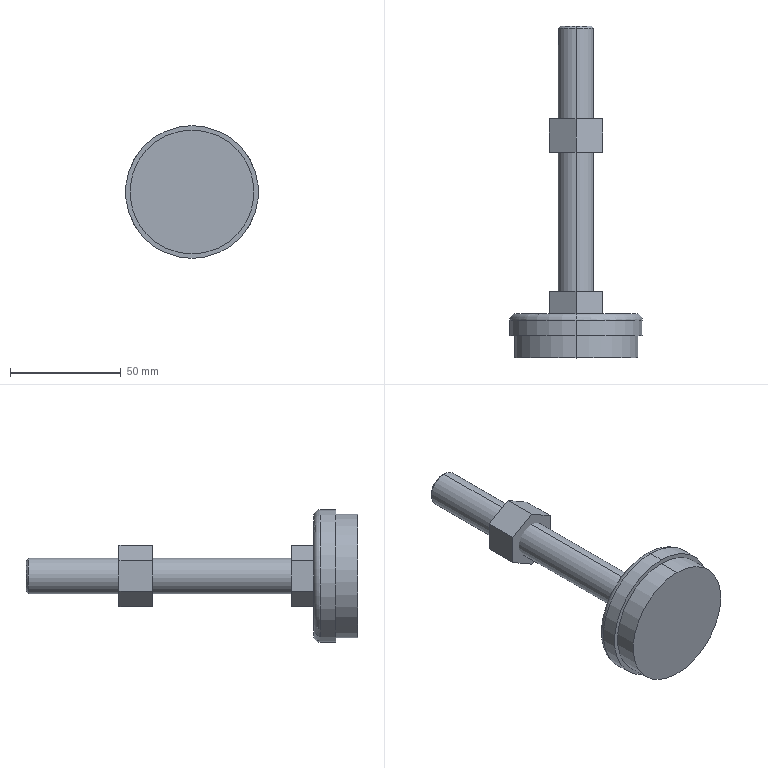Part | SolidWorks | features ICE 2, Chamfer 1, Revolution 1 | 3 solids | 32 faces | box 60 x 150 x 60 mm | volume 89123 mm3 | plane 20 | cylinder 8 | cone 2 | torus 2 | commonest cylinder face diameters 16 x4 56 x2 60 x2
STEP:
#1=CARTESIAN_POINT('',(0.,150.,7.));
#2=VERTEX_POINT('',#1);
#3=CARTESIAN_POINT('',(0.,150.,-7.));
#4=VERTEX_POINT('',#3);
#5=CARTESIAN_POINT('',(0.,150.,0.));
#6=DIRECTION('',(0.,1.,0.));
#7=DIRECTION('',(0.,0.,1.));
#8=AXIS2_PLACEMENT_3D('',#5,#6,#7);
#9=CIRCLE('',#8,7.);
#10=EDGE_CURVE('',#2,#4,#9,.T.);
#11=ORIENTED_EDGE('',*,*,#10,.F.);
#12=CARTESIAN_POINT('',(0.,149.,8.));
#13=VERTEX_POINT('',#12);
#14=CARTESIAN_POINT('',(0.,149.,8.));
#15=DIRECTION('',(0.,-0.7071,0.7071));
#16=VECTOR('',#15,1000.);
#17=LINE('',#14,#16);
#18=EDGE_CURVE('',#2,#13,#17,.T.);
#19=ORIENTED_EDGE('',*,*,#18,.T.);
#20=CARTESIAN_POINT('',(0.,149.,-8.));
#21=VERTEX_POINT('',#20);
#22=CARTESIAN_POINT('',(0.,149.,0.));
#23=DIRECTION('',(0.,-1.,0.));
#24=DIRECTION('',(0.,0.,1.));
#25=AXIS2_PLACEMENT_3D('',#22,#23,#24);
#26=CIRCLE('',#25,8.);
#27=EDGE_CURVE('',#21,#13,#26,.T.);
#28=ORIENTED_EDGE('',*,*,#27,.F.);
#29=CARTESIAN_POINT('',(0.,149.,-8.));
#30=DIRECTION('',(0.,-0.7071,-0.7071));
#31=VECTOR('',#30,1000.);
#32=LINE('',#29,#31);
#33=EDGE_CURVE('',#4,#21,#32,.T.);
#34=ORIENTED_EDGE('',*,*,#33,.F.);
#35=EDGE_LOOP('',(#11,#19,#28,#34));
#36=FACE_OUTER_BOUND('',#35,.T.);
#37=CARTESIAN_POINT('',(0.,149.,0.));
#38=DIRECTION('',(0.,-1.,0.));
#39=DIRECTION('',(0.,0.,-1.));
#40=AXIS2_PLACEMENT_3D('',#37,#38,#39);
#41=CONICAL_SURFACE('',#40,8.,0.7854);
#42=ADVANCED_FACE('',(#36),#41,.T.);
#43=CARTESIAN_POINT('',(0.,10.,-28.));
#44=VERTEX_POINT('',#43);
#45=CARTESIAN_POINT('',(0.,10.,28.));
#46=VERTEX_POINT('',#45);
#47=CARTESIAN_POINT('',(0.,10.,0.));
#48=DIRECTION('',(0.,-1.,0.));
#49=DIRECTION('',(0.,0.,-1.));
#50=AXIS2_PLACEMENT_3D('',#47,#48,#49);
#51=CIRCLE('',#50,28.);
#52=EDGE_CURVE('',#44,#46,#51,.T.);
#53=ORIENTED_EDGE('',*,*,#52,.T.);
#54=CARTESIAN_POINT('',(0.,0.,28.));
#55=VERTEX_POINT('',#54);
#56=CARTESIAN_POINT('',(0.,0.,28.));
#57=DIRECTION('',(0.,-1.,0.));
#58=VECTOR('',#57,1000.);
#59=LINE('',#56,#58);
#60=EDGE_CURVE('',#46,#55,#59,.T.);
#61=ORIENTED_EDGE('',*,*,#60,.T.);
#62=CARTESIAN_POINT('',(0.,0.,-28.));
#63=VERTEX_POINT('',#62);
#64=CARTESIAN_POINT('',(0.,0.,0.));
#65=DIRECTION('',(0.,-1.,0.));
#66=DIRECTION('',(0.,0.,-1.));
#67=AXIS2_PLACEMENT_3D('',#64,#65,#66);
#68=CIRCLE('',#67,28.);
#69=EDGE_CURVE('',#63,#55,#68,.T.);
#70=ORIENTED_EDGE('',*,*,#69,.F.);
#71=CARTESIAN_POINT('',(0.,0.,-28.));
#72=DIRECTION('',(0.,-1.,0.));
#73=VECTOR('',#72,1000.);
#74=LINE('',#71,#73);
#75=EDGE_CURVE('',#44,#63,#74,.T.);
#76=ORIENTED_EDGE('',*,*,#75,.F.);
#77=EDGE_LOOP('',(#53,#61,#70,#76));
#78=FACE_OUTER_BOUND('',#77,.T.);
#79=CARTESIAN_POINT('',(0.,0.,0.));
#80=DIRECTION('',(0.,-1.,0.));
#81=DIRECTION('',(0.,0.,-1.));
#82=AXIS2_PLACEMENT_3D('',#79,#80,#81);
#83=CYLINDRICAL_SURFACE('',#82,28.);
#84=ADVANCED_FACE('',(#78),#83,.T.);
#85=CARTESIAN_POINT('',(0.,17.,-30.));
#86=VERTEX_POINT('',#85);
#87=CARTESIAN_POINT('',(0.,17.,30.));
#88=VERTEX_POINT('',#87);
#89=CARTESIAN_POINT('',(0.,17.,0.));
#90=DIRECTION('',(0.,-1.,0.));
#91=DIRECTION('',(0.,0.,-1.));
#92=AXIS2_PLACEMENT_3D('',#89,#90,#91);
#93=CIRCLE('',#92,30.);
#94=EDGE_CURVE('',#86,#88,#93,.T.);
#95=ORIENTED_EDGE('',*,*,#94,.T.);
#96=CARTESIAN_POINT('',(0.,10.,30.));
#97=VERTEX_POINT('',#96);
#98=CARTESIAN_POINT('',(0.,0.,30.));
#99=DIRECTION('',(0.,-1.,0.));
#100=VECTOR('',#99,1000.);
#101=LINE('',#98,#100);
#102=EDGE_CURVE('',#88,#97,#101,.T.);
#103=ORIENTED_EDGE('',*,*,#102,.T.);
#104=CARTESIAN_POINT('',(0.,10.,-30.));
#105=VERTEX_POINT('',#104);
#106=CARTESIAN_POINT('',(0.,10.,0.));
#107=DIRECTION('',(0.,-1.,0.));
#108=DIRECTION('',(0.,0.,-1.));
#109=AXIS2_PLACEMENT_3D('',#106,#107,#108);
#110=CIRCLE('',#109,30.);
#111=EDGE_CURVE('',#105,#97,#110,.T.);
#112=ORIENTED_EDGE('',*,*,#111,.F.);
#113=CARTESIAN_POINT('',(0.,0.,-30.));
#114=DIRECTION('',(0.,-1.,0.));
#115=VECTOR('',#114,1000.);
#116=LINE('',#113,#115);
#117=EDGE_CURVE('',#86,#105,#116,.T.);
#118=ORIENTED_EDGE('',*,*,#117,.F.);
#119=EDGE_LOOP('',(#95,#103,#112,#118));
#120=FACE_OUTER_BOUND('',#119,.T.);
#121=CARTESIAN_POINT('',(0.,0.,0.));
#122=DIRECTION('',(0.,-1.,0.));
#123=DIRECTION('',(0.,0.,-1.));
#124=AXIS2_PLACEMENT_3D('',#121,#122,#123);
#125=CYLINDRICAL_SURFACE('',#124,30.);
#126=ADVANCED_FACE('',(#120),#125,.T.);
#127=CARTESIAN_POINT('',(0.,20.,-27.));
#128=VERTEX_POINT('',#127);
#129=CARTESIAN_POINT('',(0.,20.,27.));
#130=VERTEX_POINT('',#129);
#131=CARTESIAN_POINT('',(0.,20.,0.));
#132=DIRECTION('',(0.,-1.,0.));
#133=DIRECTION('',(0.,0.,-1.));
#134=AXIS2_PLACEMENT_3D('',#131,#132,#133);
#135=CIRCLE('',#134,27.);
#136=EDGE_CURVE('',#128,#130,#135,.T.);
#137=ORIENTED_EDGE('',*,*,#136,.T.);
#138=CARTESIAN_POINT('',(0.,17.,27.));
#139=DIRECTION('',(1.,0.,0.));
#140=DIRECTION('',(0.,0.,-1.));
#141=AXIS2_PLACEMENT_3D('',#138,#139,#140);
#142=CIRCLE('',#141,3.);
#143=EDGE_CURVE('',#130,#88,#142,.T.);
#144=ORIENTED_EDGE('',*,*,#143,.T.);
#145=ORIENTED_EDGE('',*,*,#94,.F.);
#146=CARTESIAN_POINT('',(0.,17.,-27.));
#147=DIRECTION('',(-1.,0.,0.));
#148=DIRECTION('',(0.,0.,1.));
#149=AXIS2_PLACEMENT_3D('',#146,#147,#148);
#150=CIRCLE('',#149,3.);
#151=EDGE_CURVE('',#128,#86,#150,.T.);
#152=ORIENTED_EDGE('',*,*,#151,.F.);
#153=EDGE_LOOP('',(#137,#144,#145,#152));
#154=FACE_OUTER_BOUND('',#153,.T.);
#155=CARTESIAN_POINT('',(0.,17.,0.));
#156=DIRECTION('',(0.,-1.,0.));
#157=DIRECTION('',(0.,0.,-1.));
#158=AXIS2_PLACEMENT_3D('',#155,#156,#157);
#159=TOROIDAL_SURFACE('',#158,27.,3.);
#160=ADVANCED_FACE('',(#154),#159,.T.);
#161=ORIENTED_EDGE('',*,*,#27,.T.);
#162=CARTESIAN_POINT('',(0.,20.,8.));
#163=VERTEX_POINT('',#162);
#164=CARTESIAN_POINT('',(0.,0.,8.));
#165=DIRECTION('',(0.,-1.,0.));
#166=VECTOR('',#165,1000.);
#167=LINE('',#164,#166);
#168=EDGE_CURVE('',#13,#163,#167,.T.);
#169=ORIENTED_EDGE('',*,*,#168,.T.);
#170=CARTESIAN_POINT('',(0.,20.,-8.));
#171=VERTEX_POINT('',#170);
#172=CARTESIAN_POINT('',(0.,20.,0.));
#173=DIRECTION('',(0.,-1.,0.));
#174=DIRECTION('',(0.,0.,-1.));
#175=AXIS2_PLACEMENT_3D('',#172,#173,#174);
#176=CIRCLE('',#175,8.);
#177=EDGE_CURVE('',#171,#163,#176,.T.);
#178=ORIENTED_EDGE('',*,*,#177,.F.);
#179=CARTESIAN_POINT('',(0.,0.,-8.));
#180=DIRECTION('',(0.,-1.,0.));
#181=VECTOR('',#180,1000.);
#182=LINE('',#179,#181);
#183=EDGE_CURVE('',#21,#171,#182,.T.);
#184=ORIENTED_EDGE('',*,*,#183,.F.);
#185=EDGE_LOOP('',(#161,#169,#178,#184));
#186=FACE_OUTER_BOUND('',#185,.T.);
#187=CARTESIAN_POINT('',(0.,0.,0.));
#188=DIRECTION('',(0.,-1.,0.));
#189=DIRECTION('',(0.,0.,-1.));
#190=AXIS2_PLACEMENT_3D('',#187,#188,#189);
#191=CYLINDRICAL_SURFACE('',#190,8.);
#192=ADVANCED_FACE('',(#186),#191,.T.);
#193=ORIENTED_EDGE('',*,*,#69,.T.);
#194=CARTESIAN_POINT('',(0.,0.,0.));
#195=DIRECTION('',(0.,-1.,0.));
#196=DIRECTION('',(0.,0.,-1.));
#197=AXIS2_PLACEMENT_3D('',#194,#195,#196);
#198=CIRCLE('',#197,28.);
#199=EDGE_CURVE('',#55,#63,#198,.T.);
#200=ORIENTED_EDGE('',*,*,#199,.T.);
#201=EDGE_LOOP('',(#193,#200));
#202=FACE_OUTER_BOUND('',#201,.T.);
#203=CARTESIAN_POINT('',(28.,0.,0.));
#204=DIRECTION('',(0.,-1.,0.));
#205=DIRECTION('',(0.,0.,-1.));
#206=AXIS2_PLACEMENT_3D('',#203,#204,#205);
#207=PLANE('',#206);
#208=ADVANCED_FACE('',(#202),#207,.T.);
#209=CARTESIAN_POINT('',(0.,150.,0.));
#210=DIRECTION('',(0.,1.,0.));
#211=DIRECTION('',(0.,0.,1.));
#212=AXIS2_PLACEMENT_3D('',#209,#210,#211);
#213=CIRCLE('',#212,7.);
#214=EDGE_CURVE('',#4,#2,#213,.T.);
#215=ORIENTED_EDGE('',*,*,#214,.T.);
#216=ORIENTED_EDGE('',*,*,#10,.T.);
#217=EDGE_LOOP('',(#215,#216));
#218=FACE_OUTER_BOUND('',#217,.T.);
#219=CARTESIAN_POINT('',(0.,150.,0.));
#220=DIRECTION('',(0.,1.,0.));
#221=DIRECTION('',(0.,0.,1.));
#222=AXIS2_PLACEMENT_3D('',#219,#220,#221);
#223=PLANE('',#222);
#224=ADVANCED_FACE('',(#218),#223,.T.);
#225=ORIENTED_EDGE('',*,*,#168,.F.);
#226=CARTESIAN_POINT('',(0.,149.,0.));
#227=DIRECTION('',(0.,-1.,0.));
#228=DIRECTION('',(0.,0.,1.));
#229=AXIS2_PLACEMENT_3D('',#226,#227,#228);
#230=CIRCLE('',#229,8.);
#231=EDGE_CURVE('',#13,#21,#230,.T.);
#232=ORIENTED_EDGE('',*,*,#231,.T.);
#233=ORIENTED_EDGE('',*,*,#183,.T.);
#234=CARTESIAN_POINT('',(0.,20.,0.));
#235=DIRECTION('',(0.,-1.,0.));
#236=DIRECTION('',(0.,0.,-1.));
#237=AXIS2_PLACEMENT_3D('',#234,#235,#236);
#238=CIRCLE('',#237,8.);
#239=EDGE_CURVE('',#163,#171,#238,.T.);
#240=ORIENTED_EDGE('',*,*,#239,.F.);
#241=EDGE_LOOP('',(#225,#232,#233,#240));
#242=FACE_OUTER_BOUND('',#241,.T.);
#243=CARTESIAN_POINT('',(0.,0.,0.));
#244=DIRECTION('',(0.,-1.,0.));
#245=DIRECTION('',(0.,0.,-1.));
#246=AXIS2_PLACEMENT_3D('',#243,#244,#245);
#247=CYLINDRICAL_SURFACE('',#246,8.);
#248=ADVANCED_FACE('',(#242),#247,.T.);
#249=ORIENTED_EDGE('',*,*,#177,.T.);
#250=ORIENTED_EDGE('',*,*,#239,.T.);
#251=EDGE_LOOP('',(#249,#250));
#252=FACE_BOUND('',#251,.T.);
#253=ORIENTED_EDGE('',*,*,#136,.F.);
#254=CARTESIAN_POINT('',(0.,20.,0.));
#255=DIRECTION('',(0.,-1.,0.));
#256=DIRECTION('',(0.,0.,-1.));
#257=AXIS2_PLACEMENT_3D('',#254,#255,#256);
#258=CIRCLE('',#257,27.);
#259=EDGE_CURVE('',#130,#128,#258,.T.);
#260=ORIENTED_EDGE('',*,*,#259,.F.);
#261=EDGE_LOOP('',(#253,#260));
#262=FACE_OUTER_BOUND('',#261,.T.);
#263=CARTESIAN_POINT('',(8.,20.,0.));
#264=DIRECTION('',(0.,1.,0.));
#265=DIRECTION('',(0.,0.,1.));
#266=AXIS2_PLACEMENT_3D('',#263,#264,#265);
#267=PLANE('',#266);
#268=ADVANCED_FACE('',(#252,#262),#267,.T.);
#269=ORIENTED_EDGE('',*,*,#143,.F.);
#270=ORIENTED_EDGE('',*,*,#259,.T.);
#271=ORIENTED_EDGE('',*,*,#151,.T.);
#272=CARTESIAN_POINT('',(0.,17.,0.));
#273=DIRECTION('',(0.,-1.,0.));
#274=DIRECTION('',(0.,0.,-1.));
#275=AXIS2_PLACEMENT_3D('',#272,#273,#274);
#276=CIRCLE('',#275,30.);
#277=EDGE_CURVE('',#88,#86,#276,.T.);
#278=ORIENTED_EDGE('',*,*,#277,.F.);
#279=EDGE_LOOP('',(#269,#270,#271,#278));
#280=FACE_OUTER_BOUND('',#279,.T.);
#281=CARTESIAN_POINT('',(0.,17.,0.));
#282=DIRECTION('',(0.,-1.,0.));
#283=DIRECTION('',(0.,0.,-1.));
#284=AXIS2_PLACEMENT_3D('',#281,#282,#283);
#285=TOROIDAL_SURFACE('',#284,27.,3.);
#286=ADVANCED_FACE('',(#280),#285,.T.);
#287=ORIENTED_EDGE('',*,*,#102,.F.);
#288=ORIENTED_EDGE('',*,*,#277,.T.);
#289=ORIENTED_EDGE('',*,*,#117,.T.);
#290=CARTESIAN_POINT('',(0.,10.,0.));
#291=DIRECTION('',(0.,-1.,0.));
#292=DIRECTION('',(0.,0.,-1.));
#293=AXIS2_PLACEMENT_3D('',#290,#291,#292);
#294=CIRCLE('',#293,30.);
#295=EDGE_CURVE('',#97,#105,#294,.T.);
#296=ORIENTED_EDGE('',*,*,#295,.F.);
#297=EDGE_LOOP('',(#287,#288,#289,#296));
#298=FACE_OUTER_BOUND('',#297,.T.);
#299=CARTESIAN_POINT('',(0.,0.,0.));
#300=DIRECTION('',(0.,-1.,0.));
#301=DIRECTION('',(0.,0.,-1.));
#302=AXIS2_PLACEMENT_3D('',#299,#300,#301);
#303=CYLINDRICAL_SURFACE('',#302,30.);
#304=ADVANCED_FACE('',(#298),#303,.T.);
#305=ORIENTED_EDGE('',*,*,#111,.T.);
#306=ORIENTED_EDGE('',*,*,#295,.T.);
#307=EDGE_LOOP('',(#305,#306));
#308=FACE_OUTER_BOUND('',#307,.T.);
#309=ORIENTED_EDGE('',*,*,#52,.F.);
#310=CARTESIAN_POINT('',(0.,10.,0.));
#311=DIRECTION('',(0.,-1.,0.));
#312=DIRECTION('',(0.,0.,-1.));
#313=AXIS2_PLACEMENT_3D('',#310,#311,#312);
#314=CIRCLE('',#313,28.);
#315=EDGE_CURVE('',#46,#44,#314,.T.);
#316=ORIENTED_EDGE('',*,*,#315,.F.);
#317=EDGE_LOOP('',(#309,#316));
#318=FACE_BOUND('',#317,.T.);
#319=CARTESIAN_POINT('',(30.,10.,0.));
#320=DIRECTION('',(0.,-1.,0.));
#321=DIRECTION('',(0.,0.,-1.));
#322=AXIS2_PLACEMENT_3D('',#319,#320,#321);
#323=PLANE('',#322);
#324=ADVANCED_FACE('',(#308,#318),#323,.T.);
#325=ORIENTED_EDGE('',*,*,#60,.F.);
#326=ORIENTED_EDGE('',*,*,#315,.T.);
#327=ORIENTED_EDGE('',*,*,#75,.T.);
#328=ORIENTED_EDGE('',*,*,#199,.F.);
#329=EDGE_LOOP('',(#325,#326,#327,#328));
#330=FACE_OUTER_BOUND('',#329,.T.);
#331=CARTESIAN_POINT('',(0.,0.,0.));
#332=DIRECTION('',(0.,-1.,0.));
#333=DIRECTION('',(0.,0.,-1.));
#334=AXIS2_PLACEMENT_3D('',#331,#332,#333);
#335=CYLINDRICAL_SURFACE('',#334,28.);
#336=ADVANCED_FACE('',(#330),#335,.T.);
#337=ORIENTED_EDGE('',*,*,#18,.F.);
#338=ORIENTED_EDGE('',*,*,#214,.F.);
#339=ORIENTED_EDGE('',*,*,#33,.T.);
#340=ORIENTED_EDGE('',*,*,#231,.F.);
#341=EDGE_LOOP('',(#337,#338,#339,#340));
#342=FACE_OUTER_BOUND('',#341,.T.);
#343=CARTESIAN_POINT('',(0.,149.,0.));
#344=DIRECTION('',(0.,-1.,0.));
#345=DIRECTION('',(0.,0.,-1.));
#346=AXIS2_PLACEMENT_3D('',#343,#344,#345);
#347=CONICAL_SURFACE('',#346,8.,0.7854);
#348=ADVANCED_FACE('',(#342),#347,.T.);
#349=CLOSED_SHELL('',(#42,#84,#126,#160,#192,#208,#224,#248,#268,#286,#304,#324,#336,#348));
#350=MANIFOLD_SOLID_BREP('',#349);
#351=CARTESIAN_POINT('',(0.,30.,-8.));
#352=VERTEX_POINT('',#351);
#353=CARTESIAN_POINT('',(0.,30.,8.));
#354=VERTEX_POINT('',#353);
#355=CARTESIAN_POINT('',(0.,30.,0.));
#356=DIRECTION('',(0.,1.,0.));
#357=DIRECTION('',(0.,0.,1.));
#358=AXIS2_PLACEMENT_3D('',#355,#356,#357);
#359=CIRCLE('',#358,8.);
#360=EDGE_CURVE('',#352,#354,#359,.T.);
#361=ORIENTED_EDGE('',*,*,#360,.T.);
#362=CARTESIAN_POINT('',(0.,20.,8.));
#363=VERTEX_POINT('',#362);
#364=CARTESIAN_POINT('',(0.,30.,8.));
#365=DIRECTION('',(0.,-1.,0.));
#366=VECTOR('',#365,1000.);
#367=LINE('',#364,#366);
#368=EDGE_CURVE('',#354,#363,#367,.T.);
#369=ORIENTED_EDGE('',*,*,#368,.T.);
#370=CARTESIAN_POINT('',(0.,20.,-8.));
#371=VERTEX_POINT('',#370);
#372=CARTESIAN_POINT('',(0.,20.,0.));
#373=DIRECTION('',(0.,1.,0.));
#374=DIRECTION('',(0.,0.,1.));
#375=AXIS2_PLACEMENT_3D('',#372,#373,#374);
#376=CIRCLE('',#375,8.);
#377=EDGE_CURVE('',#371,#363,#376,.T.);
#378=ORIENTED_EDGE('',*,*,#377,.F.);
#379=CARTESIAN_POINT('',(0.,30.,-8.));
#380=DIRECTION('',(0.,-1.,0.));
#381=VECTOR('',#380,1000.);
#382=LINE('',#379,#381);
#383=EDGE_CURVE('',#352,#371,#382,.T.);
#384=ORIENTED_EDGE('',*,*,#383,.F.);
#385=EDGE_LOOP('',(#361,#369,#378,#384));
#386=FACE_OUTER_BOUND('',#385,.T.);
#387=CARTESIAN_POINT('',(0.,30.,0.));
#388=DIRECTION('',(0.,-1.,0.));
#389=DIRECTION('',(0.,0.,-1.));
#390=AXIS2_PLACEMENT_3D('',#387,#388,#389);
#391=CYLINDRICAL_SURFACE('',#390,8.);
#392=ADVANCED_FACE('',(#386),#391,.F.);
#393=CARTESIAN_POINT('',(12.,30.,-6.928));
#394=VERTEX_POINT('',#393);
#395=CARTESIAN_POINT('',(0.,30.,-13.856));
#396=VERTEX_POINT('',#395);
#397=CARTESIAN_POINT('',(12.,30.,-6.928));
#398=DIRECTION('',(-0.866,0.,-0.5));
#399=VECTOR('',#398,1000.);
#400=LINE('',#397,#399);
#401=EDGE_CURVE('',#394,#396,#400,.T.);
#402=ORIENTED_EDGE('',*,*,#401,.T.);
#403=CARTESIAN_POINT('',(-12.,30.,-6.928));
#404=VERTEX_POINT('',#403);
#405=CARTESIAN_POINT('',(0.,30.,-13.856));
#406=DIRECTION('',(-0.866,0.,0.5));
#407=VECTOR('',#406,1000.);
#408=LINE('',#405,#407);
#409=EDGE_CURVE('',#396,#404,#408,.T.);
#410=ORIENTED_EDGE('',*,*,#409,.T.);
#411=CARTESIAN_POINT('',(-12.,30.,6.928));
#412=VERTEX_POINT('',#411);
#413=CARTESIAN_POINT('',(-12.,30.,-6.928));
#414=DIRECTION('',(0.,0.,1.));
#415=VECTOR('',#414,1000.);
#416=LINE('',#413,#415);
#417=EDGE_CURVE('',#404,#412,#416,.T.);
#418=ORIENTED_EDGE('',*,*,#417,.T.);
#419=CARTESIAN_POINT('',(0.,30.,13.856));
#420=VERTEX_POINT('',#419);
#421=CARTESIAN_POINT('',(-12.,30.,6.928));
#422=DIRECTION('',(0.866,0.,0.5));
#423=VECTOR('',#422,1000.);
#424=LINE('',#421,#423);
#425=EDGE_CURVE('',#412,#420,#424,.T.);
#426=ORIENTED_EDGE('',*,*,#425,.T.);
#427=CARTESIAN_POINT('',(12.,30.,6.928));
#428=VERTEX_POINT('',#427);
#429=CARTESIAN_POINT('',(0.,30.,13.856));
#430=DIRECTION('',(0.866,0.,-0.5));
#431=VECTOR('',#430,1000.);
#432=LINE('',#429,#431);
#433=EDGE_CURVE('',#420,#428,#432,.T.);
#434=ORIENTED_EDGE('',*,*,#433,.T.);
#435=CARTESIAN_POINT('',(12.,30.,6.928));
#436=DIRECTION('',(0.,0.,-1.));
#437=VECTOR('',#436,1000.);
#438=LINE('',#435,#437);
#439=EDGE_CURVE('',#428,#394,#438,.T.);
#440=ORIENTED_EDGE('',*,*,#439,.T.);
#441=EDGE_LOOP('',(#402,#410,#418,#426,#434,#440));
#442=FACE_OUTER_BOUND('',#441,.T.);
#443=ORIENTED_EDGE('',*,*,#360,.F.);
#444=CARTESIAN_POINT('',(0.,30.,0.));
#445=DIRECTION('',(0.,1.,0.));
#446=DIRECTION('',(0.,0.,1.));
#447=AXIS2_PLACEMENT_3D('',#444,#445,#446);
#448=CIRCLE('',#447,8.);
#449=EDGE_CURVE('',#354,#352,#448,.T.);
#450=ORIENTED_EDGE('',*,*,#449,.F.);
#451=EDGE_LOOP('',(#443,#450));
#452=FACE_BOUND('',#451,.T.);
#453=CARTESIAN_POINT('',(0.,30.,0.));
#454=DIRECTION('',(0.,1.,0.));
#455=DIRECTION('',(0.,0.,1.));
#456=AXIS2_PLACEMENT_3D('',#453,#454,#455);
#457=PLANE('',#456);
#458=ADVANCED_FACE('',(#442,#452),#457,.T.);
#459=CARTESIAN_POINT('',(12.,20.,-6.928));
#460=VERTEX_POINT('',#459);
#461=CARTESIAN_POINT('',(0.,20.,-13.856));
#462=VERTEX_POINT('',#461);
#463=CARTESIAN_POINT('',(12.,20.,-6.928));
#464=DIRECTION('',(-0.866,0.,-0.5));
#465=VECTOR('',#464,1000.);
#466=LINE('',#463,#465);
#467=EDGE_CURVE('',#460,#462,#466,.T.);
#468=ORIENTED_EDGE('',*,*,#467,.F.);
#469=CARTESIAN_POINT('',(12.,20.,6.928));
#470=VERTEX_POINT('',#469);
#471=CARTESIAN_POINT('',(12.,20.,6.928));
#472=DIRECTION('',(0.,0.,-1.));
#473=VECTOR('',#472,1000.);
#474=LINE('',#471,#473);
#475=EDGE_CURVE('',#470,#460,#474,.T.);
#476=ORIENTED_EDGE('',*,*,#475,.F.);
#477=CARTESIAN_POINT('',(0.,20.,13.856));
#478=VERTEX_POINT('',#477);
#479=CARTESIAN_POINT('',(0.,20.,13.856));
#480=DIRECTION('',(0.866,0.,-0.5));
#481=VECTOR('',#480,1000.);
#482=LINE('',#479,#481);
#483=EDGE_CURVE('',#478,#470,#482,.T.);
#484=ORIENTED_EDGE('',*,*,#483,.F.);
#485=CARTESIAN_POINT('',(-12.,20.,6.928));
#486=VERTEX_POINT('',#485);
#487=CARTESIAN_POINT('',(-12.,20.,6.928));
#488=DIRECTION('',(0.866,0.,0.5));
#489=VECTOR('',#488,1000.);
#490=LINE('',#487,#489);
#491=EDGE_CURVE('',#486,#478,#490,.T.);
#492=ORIENTED_EDGE('',*,*,#491,.F.);
#493=CARTESIAN_POINT('',(-12.,20.,-6.928));
#494=VERTEX_POINT('',#493);
#495=CARTESIAN_POINT('',(-12.,20.,-6.928));
#496=DIRECTION('',(0.,0.,1.));
#497=VECTOR('',#496,1000.);
#498=LINE('',#495,#497);
#499=EDGE_CURVE('',#494,#486,#498,.T.);
#500=ORIENTED_EDGE('',*,*,#499,.F.);
#501=CARTESIAN_POINT('',(0.,20.,-13.856));
#502=DIRECTION('',(-0.866,0.,0.5));
#503=VECTOR('',#502,1000.);
#504=LINE('',#501,#503);
#505=EDGE_CURVE('',#462,#494,#504,.T.);
#506=ORIENTED_EDGE('',*,*,#505,.F.);
#507=EDGE_LOOP('',(#468,#476,#484,#492,#500,#506));
#508=FACE_OUTER_BOUND('',#507,.T.);
#509=ORIENTED_EDGE('',*,*,#377,.T.);
#510=CARTESIAN_POINT('',(0.,20.,0.));
#511=DIRECTION('',(0.,1.,0.));
#512=DIRECTION('',(0.,0.,1.));
#513=AXIS2_PLACEMENT_3D('',#510,#511,#512);
#514=CIRCLE('',#513,8.);
#515=EDGE_CURVE('',#363,#371,#514,.T.);
#516=ORIENTED_EDGE('',*,*,#515,.T.);
#517=EDGE_LOOP('',(#509,#516));
#518=FACE_BOUND('',#517,.T.);
#519=CARTESIAN_POINT('',(0.,20.,0.));
#520=DIRECTION('',(0.,1.,0.));
#521=DIRECTION('',(0.,0.,1.));
#522=AXIS2_PLACEMENT_3D('',#519,#520,#521);
#523=PLANE('',#522);
#524=ADVANCED_FACE('',(#508,#518),#523,.F.);
#525=ORIENTED_EDGE('',*,*,#467,.T.);
#526=CARTESIAN_POINT('',(0.,30.,-13.856));
#527=DIRECTION('',(0.,-1.,0.));
#528=VECTOR('',#527,1000.);
#529=LINE('',#526,#528);
#530=EDGE_CURVE('',#396,#462,#529,.T.);
#531=ORIENTED_EDGE('',*,*,#530,.F.);
#532=ORIENTED_EDGE('',*,*,#401,.F.);
#533=CARTESIAN_POINT('',(12.,30.,-6.928));
#534=DIRECTION('',(0.,-1.,0.));
#535=VECTOR('',#534,1000.);
#536=LINE('',#533,#535);
#537=EDGE_CURVE('',#394,#460,#536,.T.);
#538=ORIENTED_EDGE('',*,*,#537,.T.);
#539=EDGE_LOOP('',(#525,#531,#532,#538));
#540=FACE_OUTER_BOUND('',#539,.T.);
#541=CARTESIAN_POINT('',(12.,30.,-6.928));
#542=DIRECTION('',(-0.5,0.,0.866));
#543=DIRECTION('',(0.866,0.,0.5));
#544=AXIS2_PLACEMENT_3D('',#541,#542,#543);
#545=PLANE('',#544);
#546=ADVANCED_FACE('',(#540),#545,.F.);
#547=ORIENTED_EDGE('',*,*,#505,.T.);
#548=CARTESIAN_POINT('',(-12.,30.,-6.928));
#549=DIRECTION('',(0.,-1.,0.));
#550=VECTOR('',#549,1000.);
#551=LINE('',#548,#550);
#552=EDGE_CURVE('',#404,#494,#551,.T.);
#553=ORIENTED_EDGE('',*,*,#552,.F.);
#554=ORIENTED_EDGE('',*,*,#409,.F.);
#555=ORIENTED_EDGE('',*,*,#530,.T.);
#556=EDGE_LOOP('',(#547,#553,#554,#555));
#557=FACE_OUTER_BOUND('',#556,.T.);
#558=CARTESIAN_POINT('',(0.,30.,-13.856));
#559=DIRECTION('',(0.5,0.,0.866));
#560=DIRECTION('',(0.866,0.,-0.5));
#561=AXIS2_PLACEMENT_3D('',#558,#559,#560);
#562=PLANE('',#561);
#563=ADVANCED_FACE('',(#557),#562,.F.);
#564=ORIENTED_EDGE('',*,*,#499,.T.);
#565=CARTESIAN_POINT('',(-12.,30.,6.928));
#566=DIRECTION('',(0.,-1.,0.));
#567=VECTOR('',#566,1000.);
#568=LINE('',#565,#567);
#569=EDGE_CURVE('',#412,#486,#568,.T.);
#570=ORIENTED_EDGE('',*,*,#569,.F.);
#571=ORIENTED_EDGE('',*,*,#417,.F.);
#572=ORIENTED_EDGE('',*,*,#552,.T.);
#573=EDGE_LOOP('',(#564,#570,#571,#572));
#574=FACE_OUTER_BOUND('',#573,.T.);
#575=CARTESIAN_POINT('',(-12.,30.,-6.928));
#576=DIRECTION('',(1.,0.,0.));
#577=DIRECTION('',(0.,0.,-1.));
#578=AXIS2_PLACEMENT_3D('',#575,#576,#577);
#579=PLANE('',#578);
#580=ADVANCED_FACE('',(#574),#579,.F.);
#581=ORIENTED_EDGE('',*,*,#491,.T.);
#582=CARTESIAN_POINT('',(0.,30.,13.856));
#583=DIRECTION('',(0.,-1.,0.));
#584=VECTOR('',#583,1000.);
#585=LINE('',#582,#584);
#586=EDGE_CURVE('',#420,#478,#585,.T.);
#587=ORIENTED_EDGE('',*,*,#586,.F.);
#588=ORIENTED_EDGE('',*,*,#425,.F.);
#589=ORIENTED_EDGE('',*,*,#569,.T.);
#590=EDGE_LOOP('',(#581,#587,#588,#589));
#591=FACE_OUTER_BOUND('',#590,.T.);
#592=CARTESIAN_POINT('',(-12.,30.,6.928));
#593=DIRECTION('',(0.5,0.,-0.866));
#594=DIRECTION('',(-0.866,0.,-0.5));
#595=AXIS2_PLACEMENT_3D('',#592,#593,#594);
#596=PLANE('',#595);
#597=ADVANCED_FACE('',(#591),#596,.F.);
#598=ORIENTED_EDGE('',*,*,#483,.T.);
#599=CARTESIAN_POINT('',(12.,30.,6.928));
#600=DIRECTION('',(0.,-1.,0.));
#601=VECTOR('',#600,1000.);
#602=LINE('',#599,#601);
#603=EDGE_CURVE('',#428,#470,#602,.T.);
#604=ORIENTED_EDGE('',*,*,#603,.F.);
#605=ORIENTED_EDGE('',*,*,#433,.F.);
#606=ORIENTED_EDGE('',*,*,#586,.T.);
#607=EDGE_LOOP('',(#598,#604,#605,#606));
#608=FACE_OUTER_BOUND('',#607,.T.);
#609=CARTESIAN_POINT('',(0.,30.,13.856));
#610=DIRECTION('',(-0.5,0.,-0.866));
#611=DIRECTION('',(-0.866,0.,0.5));
#612=AXIS2_PLACEMENT_3D('',#609,#610,#611);
#613=PLANE('',#612);
#614=ADVANCED_FACE('',(#608),#613,.F.);
#615=ORIENTED_EDGE('',*,*,#475,.T.);
#616=ORIENTED_EDGE('',*,*,#537,.F.);
#617=ORIENTED_EDGE('',*,*,#439,.F.);
#618=ORIENTED_EDGE('',*,*,#603,.T.);
#619=EDGE_LOOP('',(#615,#616,#617,#618));
#620=FACE_OUTER_BOUND('',#619,.T.);
#621=CARTESIAN_POINT('',(12.,30.,6.928));
#622=DIRECTION('',(-1.,0.,0.));
#623=DIRECTION('',(0.,0.,1.));
#624=AXIS2_PLACEMENT_3D('',#621,#622,#623);
#625=PLANE('',#624);
#626=ADVANCED_FACE('',(#620),#625,.F.);
#627=ORIENTED_EDGE('',*,*,#368,.F.);
#628=ORIENTED_EDGE('',*,*,#449,.T.);
#629=ORIENTED_EDGE('',*,*,#383,.T.);
#630=ORIENTED_EDGE('',*,*,#515,.F.);
#631=EDGE_LOOP('',(#627,#628,#629,#630));
#632=FACE_OUTER_BOUND('',#631,.T.);
#633=CARTESIAN_POINT('',(0.,30.,0.));
#634=DIRECTION('',(0.,-1.,0.));
#635=DIRECTION('',(0.,0.,-1.));
#636=AXIS2_PLACEMENT_3D('',#633,#634,#635);
#637=CYLINDRICAL_SURFACE('',#636,8.);
#638=ADVANCED_FACE('',(#632),#637,.F.);
#639=CLOSED_SHELL('',(#392,#458,#524,#546,#563,#580,#597,#614,#626,#638));
#640=MANIFOLD_SOLID_BREP('',#639);
#641=CARTESIAN_POINT('',(12.,93.,6.928));
#642=VERTEX_POINT('',#641);
#643=CARTESIAN_POINT('',(12.,93.,-6.928));
#644=VERTEX_POINT('',#643);
#645=CARTESIAN_POINT('',(12.,93.,6.928));
#646=DIRECTION('',(0.,0.,-1.));
#647=VECTOR('',#646,1000.);
#648=LINE('',#645,#647);
#649=EDGE_CURVE('',#642,#644,#648,.T.);
#650=ORIENTED_EDGE('',*,*,#649,.T.);
#651=CARTESIAN_POINT('',(12.,108.,-6.928));
#652=VERTEX_POINT('',#651);
#653=CARTESIAN_POINT('',(12.,108.,-6.928));
#654=DIRECTION('',(0.,-1.,0.));
#655=VECTOR('',#654,1000.);
#656=LINE('',#653,#655);
#657=EDGE_CURVE('',#652,#644,#656,.T.);
#658=ORIENTED_EDGE('',*,*,#657,.F.);
#659=CARTESIAN_POINT('',(12.,108.,6.928));
#660=VERTEX_POINT('',#659);
#661=CARTESIAN_POINT('',(12.,108.,6.928));
#662=DIRECTION('',(0.,0.,-1.));
#663=VECTOR('',#662,1000.);
#664=LINE('',#661,#663);
#665=EDGE_CURVE('',#660,#652,#664,.T.);
#666=ORIENTED_EDGE('',*,*,#665,.F.);
#667=CARTESIAN_POINT('',(12.,108.,6.928));
#668=DIRECTION('',(0.,-1.,0.));
#669=VECTOR('',#668,1000.);
#670=LINE('',#667,#669);
#671=EDGE_CURVE('',#660,#642,#670,.T.);
#672=ORIENTED_EDGE('',*,*,#671,.T.);
#673=EDGE_LOOP('',(#650,#658,#666,#672));
#674=FACE_OUTER_BOUND('',#673,.T.);
#675=CARTESIAN_POINT('',(12.,108.,6.928));
#676=DIRECTION('',(-1.,0.,0.));
#677=DIRECTION('',(0.,0.,1.));
#678=AXIS2_PLACEMENT_3D('',#675,#676,#677);
#679=PLANE('',#678);
#680=ADVANCED_FACE('',(#674),#679,.F.);
#681=CARTESIAN_POINT('',(0.,93.,-13.856));
#682=VERTEX_POINT('',#681);
#683=CARTESIAN_POINT('',(12.,93.,-6.928));
#684=DIRECTION('',(-0.866,0.,-0.5));
#685=VECTOR('',#684,1000.);
#686=LINE('',#683,#685);
#687=EDGE_CURVE('',#644,#682,#686,.T.);
#688=ORIENTED_EDGE('',*,*,#687,.T.);
#689=CARTESIAN_POINT('',(0.,108.,-13.856));
#690=VERTEX_POINT('',#689);
#691=CARTESIAN_POINT('',(0.,108.,-13.856));
#692=DIRECTION('',(0.,-1.,0.));
#693=VECTOR('',#692,1000.);
#694=LINE('',#691,#693);
#695=EDGE_CURVE('',#690,#682,#694,.T.);
#696=ORIENTED_EDGE('',*,*,#695,.F.);
#697=CARTESIAN_POINT('',(12.,108.,-6.928));
#698=DIRECTION('',(-0.866,0.,-0.5));
#699=VECTOR('',#698,1000.);
#700=LINE('',#697,#699);
#701=EDGE_CURVE('',#652,#690,#700,.T.);
#702=ORIENTED_EDGE('',*,*,#701,.F.);
#703=ORIENTED_EDGE('',*,*,#657,.T.);
#704=EDGE_LOOP('',(#688,#696,#702,#703));
#705=FACE_OUTER_BOUND('',#704,.T.);
#706=CARTESIAN_POINT('',(12.,108.,-6.928));
#707=DIRECTION('',(-0.5,0.,0.866));
#708=DIRECTION('',(0.866,0.,0.5));
#709=AXIS2_PLACEMENT_3D('',#706,#707,#708);
#710=PLANE('',#709);
#711=ADVANCED_FACE('',(#705),#710,.F.);
#712=CARTESIAN_POINT('',(-12.,93.,-6.928));
#713=VERTEX_POINT('',#712);
#714=CARTESIAN_POINT('',(0.,93.,-13.856));
#715=DIRECTION('',(-0.866,0.,0.5));
#716=VECTOR('',#715,1000.);
#717=LINE('',#714,#716);
#718=EDGE_CURVE('',#682,#713,#717,.T.);
#719=ORIENTED_EDGE('',*,*,#718,.T.);
#720=CARTESIAN_POINT('',(-12.,108.,-6.928));
#721=VERTEX_POINT('',#720);
#722=CARTESIAN_POINT('',(-12.,108.,-6.928));
#723=DIRECTION('',(0.,-1.,0.));
#724=VECTOR('',#723,1000.);
#725=LINE('',#722,#724);
#726=EDGE_CURVE('',#721,#713,#725,.T.);
#727=ORIENTED_EDGE('',*,*,#726,.F.);
#728=CARTESIAN_POINT('',(0.,108.,-13.856));
#729=DIRECTION('',(-0.866,0.,0.5));
#730=VECTOR('',#729,1000.);
#731=LINE('',#728,#730);
#732=EDGE_CURVE('',#690,#721,#731,.T.);
#733=ORIENTED_EDGE('',*,*,#732,.F.);
#734=ORIENTED_EDGE('',*,*,#695,.T.);
#735=EDGE_LOOP('',(#719,#727,#733,#734));
#736=FACE_OUTER_BOUND('',#735,.T.);
#737=CARTESIAN_POINT('',(0.,108.,-13.856));
#738=DIRECTION('',(0.5,0.,0.866));
#739=DIRECTION('',(0.866,0.,-0.5));
#740=AXIS2_PLACEMENT_3D('',#737,#738,#739);
#741=PLANE('',#740);
#742=ADVANCED_FACE('',(#736),#741,.F.);
#743=CARTESIAN_POINT('',(-12.,93.,6.928));
#744=VERTEX_POINT('',#743);
#745=CARTESIAN_POINT('',(-12.,93.,-6.928));
#746=DIRECTION('',(0.,0.,1.));
#747=VECTOR('',#746,1000.);
#748=LINE('',#745,#747);
#749=EDGE_CURVE('',#713,#744,#748,.T.);
#750=ORIENTED_EDGE('',*,*,#749,.T.);
#751=CARTESIAN_POINT('',(-12.,108.,6.928));
#752=VERTEX_POINT('',#751);
#753=CARTESIAN_POINT('',(-12.,108.,6.928));
#754=DIRECTION('',(0.,-1.,0.));
#755=VECTOR('',#754,1000.);
#756=LINE('',#753,#755);
#757=EDGE_CURVE('',#752,#744,#756,.T.);
#758=ORIENTED_EDGE('',*,*,#757,.F.);
#759=CARTESIAN_POINT('',(-12.,108.,-6.928));
#760=DIRECTION('',(0.,0.,1.));
#761=VECTOR('',#760,1000.);
#762=LINE('',#759,#761);
#763=EDGE_CURVE('',#721,#752,#762,.T.);
#764=ORIENTED_EDGE('',*,*,#763,.F.);
#765=ORIENTED_EDGE('',*,*,#726,.T.);
#766=EDGE_LOOP('',(#750,#758,#764,#765));
#767=FACE_OUTER_BOUND('',#766,.T.);
#768=CARTESIAN_POINT('',(-12.,108.,-6.928));
#769=DIRECTION('',(1.,0.,0.));
#770=DIRECTION('',(0.,0.,-1.));
#771=AXIS2_PLACEMENT_3D('',#768,#769,#770);
#772=PLANE('',#771);
#773=ADVANCED_FACE('',(#767),#772,.F.);
#774=CARTESIAN_POINT('',(0.,93.,13.856));
#775=VERTEX_POINT('',#774);
#776=CARTESIAN_POINT('',(-12.,93.,6.928));
#777=DIRECTION('',(0.866,0.,0.5));
#778=VECTOR('',#777,1000.);
#779=LINE('',#776,#778);
#780=EDGE_CURVE('',#744,#775,#779,.T.);
#781=ORIENTED_EDGE('',*,*,#780,.T.);
#782=CARTESIAN_POINT('',(0.,108.,13.856));
#783=VERTEX_POINT('',#782);
#784=CARTESIAN_POINT('',(0.,108.,13.856));
#785=DIRECTION('',(0.,-1.,0.));
#786=VECTOR('',#785,1000.);
#787=LINE('',#784,#786);
#788=EDGE_CURVE('',#783,#775,#787,.T.);
#789=ORIENTED_EDGE('',*,*,#788,.F.);
#790=CARTESIAN_POINT('',(-12.,108.,6.928));
#791=DIRECTION('',(0.866,0.,0.5));
#792=VECTOR('',#791,1000.);
#793=LINE('',#790,#792);
#794=EDGE_CURVE('',#752,#783,#793,.T.);
#795=ORIENTED_EDGE('',*,*,#794,.F.);
#796=ORIENTED_EDGE('',*,*,#757,.T.);
#797=EDGE_LOOP('',(#781,#789,#795,#796));
#798=FACE_OUTER_BOUND('',#797,.T.);
#799=CARTESIAN_POINT('',(-12.,108.,6.928));
#800=DIRECTION('',(0.5,0.,-0.866));
#801=DIRECTION('',(-0.866,0.,-0.5));
#802=AXIS2_PLACEMENT_3D('',#799,#800,#801);
#803=PLANE('',#802);
#804=ADVANCED_FACE('',(#798),#803,.F.);
#805=CARTESIAN_POINT('',(0.,93.,13.856));
#806=DIRECTION('',(0.866,0.,-0.5));
#807=VECTOR('',#806,1000.);
#808=LINE('',#805,#807);
#809=EDGE_CURVE('',#775,#642,#808,.T.);
#810=ORIENTED_EDGE('',*,*,#809,.T.);
#811=ORIENTED_EDGE('',*,*,#671,.F.);
#812=CARTESIAN_POINT('',(0.,108.,13.856));
#813=DIRECTION('',(0.866,0.,-0.5));
#814=VECTOR('',#813,1000.);
#815=LINE('',#812,#814);
#816=EDGE_CURVE('',#783,#660,#815,.T.);
#817=ORIENTED_EDGE('',*,*,#816,.F.);
#818=ORIENTED_EDGE('',*,*,#788,.T.);
#819=EDGE_LOOP('',(#810,#811,#817,#818));
#820=FACE_OUTER_BOUND('',#819,.T.);
#821=CARTESIAN_POINT('',(0.,108.,13.856));
#822=DIRECTION('',(-0.5,0.,-0.866));
#823=DIRECTION('',(-0.866,0.,0.5));
#824=AXIS2_PLACEMENT_3D('',#821,#822,#823);
#825=PLANE('',#824);
#826=ADVANCED_FACE('',(#820),#825,.F.);
#827=ORIENTED_EDGE('',*,*,#665,.T.);
#828=ORIENTED_EDGE('',*,*,#701,.T.);
#829=ORIENTED_EDGE('',*,*,#732,.T.);
#830=ORIENTED_EDGE('',*,*,#763,.T.);
#831=ORIENTED_EDGE('',*,*,#794,.T.);
#832=ORIENTED_EDGE('',*,*,#816,.T.);
#833=EDGE_LOOP('',(#827,#828,#829,#830,#831,#832));
#834=FACE_OUTER_BOUND('',#833,.T.);
#835=CARTESIAN_POINT('',(0.,108.,0.));
#836=DIRECTION('',(0.,1.,0.));
#837=DIRECTION('',(0.,0.,1.));
#838=AXIS2_PLACEMENT_3D('',#835,#836,#837);
#839=PLANE('',#838);
#840=ADVANCED_FACE('',(#834),#839,.T.);
#841=ORIENTED_EDGE('',*,*,#649,.F.);
#842=ORIENTED_EDGE('',*,*,#809,.F.);
#843=ORIENTED_EDGE('',*,*,#780,.F.);
#844=ORIENTED_EDGE('',*,*,#749,.F.);
#845=ORIENTED_EDGE('',*,*,#718,.F.);
#846=ORIENTED_EDGE('',*,*,#687,.F.);
#847=EDGE_LOOP('',(#841,#842,#843,#844,#845,#846));
#848=FACE_OUTER_BOUND('',#847,.T.);
#849=CARTESIAN_POINT('',(0.,93.,0.));
#850=DIRECTION('',(0.,1.,0.));
#851=DIRECTION('',(0.,0.,1.));
#852=AXIS2_PLACEMENT_3D('',#849,#850,#851);
#853=PLANE('',#852);
#854=ADVANCED_FACE('',(#848),#853,.F.);
#855=CLOSED_SHELL('',(#680,#711,#742,#773,#804,#826,#840,#854));
#856=MANIFOLD_SOLID_BREP('',#855);
#857=CARTESIAN_POINT('',(0.,0.,0.));
#858=DIRECTION('',(0.,0.,1.));
#859=DIRECTION('',(1.,0.,0.));
#860=AXIS2_PLACEMENT_3D('',#857,#858,#859);
#861=(LENGTH_UNIT()NAMED_UNIT(*)SI_UNIT(.MILLI.,.METRE.));
#862=UNCERTAINTY_MEASURE_WITH_UNIT(LENGTH_MEASURE(0.00001),#861,'','');
#863=(NAMED_UNIT(*)PLANE_ANGLE_UNIT()SI_UNIT($,.RADIAN.));
#864=(NAMED_UNIT(*)SI_UNIT($,.STERADIAN.)SOLID_ANGLE_UNIT());
#865=(GEOMETRIC_REPRESENTATION_CONTEXT(3)GLOBAL_UNCERTAINTY_ASSIGNED_CONTEXT((#862))GLOBAL_UNIT_ASSIGNED_CONTEXT((#861,#863,#864))REPRESENTATION_CONTEXT('',''));
#866=ADVANCED_BREP_SHAPE_REPRESENTATION('',(#350,#640,#856,#860),#865);